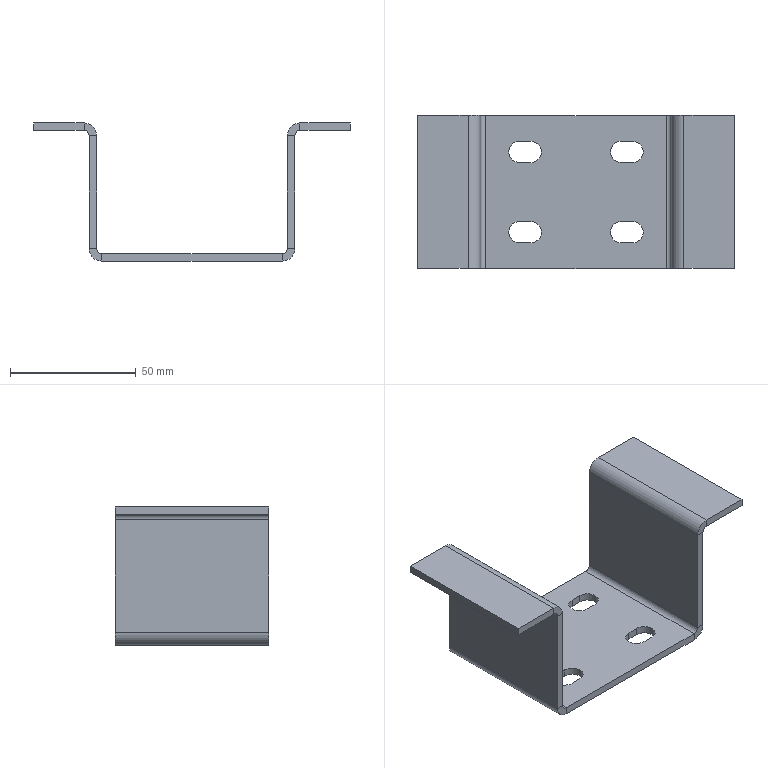Part | STEP file | Part 5 | 1 solid | 58 faces | box 126 x 61 x 55 mm | volume 39850 mm3 | plane 38 | cylinder 20 | commonest cylinder face diameters 8.5 x12 4 x4 10 x4